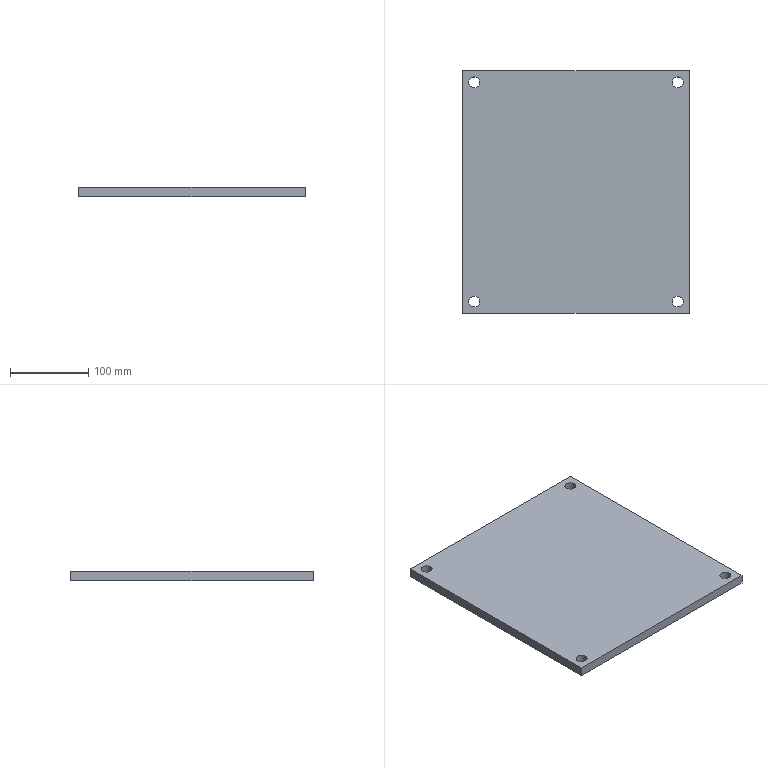Part | STEP file | X77-03027 | 1 solid | 14 faces | box 290 x 310 x 12 mm | volume 1071411 mm3 | cylinder 8 | plane 6 | commonest cylinder face diameters 14 x8
STEP:
#1=CARTESIAN_POINT('',(-3500.936,-1699.184,12.));
#2=VERTEX_POINT('',#1);
#3=CARTESIAN_POINT('',(-3514.936,-1699.184,12.));
#4=VERTEX_POINT('',#3);
#5=CARTESIAN_POINT('',(-3507.936,-1699.184,12.));
#6=DIRECTION('',(0.,0.,-1.));
#7=DIRECTION('',(-1.,0.,0.));
#8=AXIS2_PLACEMENT_3D('',#5,#6,#7);
#9=CIRCLE('',#8,7.);
#10=EDGE_CURVE('',#2,#4,#9,.T.);
#11=ORIENTED_EDGE('',*,*,#10,.F.);
#12=CARTESIAN_POINT('',(-3500.936,-1699.184,0.));
#13=VERTEX_POINT('',#12);
#14=CARTESIAN_POINT('',(-3500.936,-1699.184,0.));
#15=DIRECTION('',(0.,0.,-1.));
#16=VECTOR('',#15,1000.);
#17=LINE('',#14,#16);
#18=EDGE_CURVE('',#2,#13,#17,.T.);
#19=ORIENTED_EDGE('',*,*,#18,.T.);
#20=CARTESIAN_POINT('',(-3514.936,-1699.184,0.));
#21=VERTEX_POINT('',#20);
#22=CARTESIAN_POINT('',(-3507.936,-1699.184,0.));
#23=DIRECTION('',(0.,0.,-1.));
#24=DIRECTION('',(-1.,0.,0.));
#25=AXIS2_PLACEMENT_3D('',#22,#23,#24);
#26=CIRCLE('',#25,7.);
#27=EDGE_CURVE('',#13,#21,#26,.T.);
#28=ORIENTED_EDGE('',*,*,#27,.T.);
#29=CARTESIAN_POINT('',(-3514.936,-1699.184,0.));
#30=DIRECTION('',(0.,0.,-1.));
#31=VECTOR('',#30,1000.);
#32=LINE('',#29,#31);
#33=EDGE_CURVE('',#4,#21,#32,.T.);
#34=ORIENTED_EDGE('',*,*,#33,.F.);
#35=EDGE_LOOP('',(#11,#19,#28,#34));
#36=FACE_OUTER_BOUND('',#35,.T.);
#37=CARTESIAN_POINT('',(-3507.936,-1699.184,0.));
#38=DIRECTION('',(0.,0.,-1.));
#39=DIRECTION('',(-1.,0.,0.));
#40=AXIS2_PLACEMENT_3D('',#37,#38,#39);
#41=CYLINDRICAL_SURFACE('',#40,7.);
#42=ADVANCED_FACE('',(#36),#41,.F.);
#43=CARTESIAN_POINT('',(-3240.936,-1699.184,12.));
#44=VERTEX_POINT('',#43);
#45=CARTESIAN_POINT('',(-3254.936,-1699.184,12.));
#46=VERTEX_POINT('',#45);
#47=CARTESIAN_POINT('',(-3247.936,-1699.184,12.));
#48=DIRECTION('',(0.,0.,-1.));
#49=DIRECTION('',(-1.,0.,0.));
#50=AXIS2_PLACEMENT_3D('',#47,#48,#49);
#51=CIRCLE('',#50,7.);
#52=EDGE_CURVE('',#44,#46,#51,.T.);
#53=ORIENTED_EDGE('',*,*,#52,.F.);
#54=CARTESIAN_POINT('',(-3240.936,-1699.184,0.));
#55=VERTEX_POINT('',#54);
#56=CARTESIAN_POINT('',(-3240.936,-1699.184,0.));
#57=DIRECTION('',(0.,0.,-1.));
#58=VECTOR('',#57,1000.);
#59=LINE('',#56,#58);
#60=EDGE_CURVE('',#44,#55,#59,.T.);
#61=ORIENTED_EDGE('',*,*,#60,.T.);
#62=CARTESIAN_POINT('',(-3254.936,-1699.184,0.));
#63=VERTEX_POINT('',#62);
#64=CARTESIAN_POINT('',(-3247.936,-1699.184,0.));
#65=DIRECTION('',(0.,0.,-1.));
#66=DIRECTION('',(-1.,0.,0.));
#67=AXIS2_PLACEMENT_3D('',#64,#65,#66);
#68=CIRCLE('',#67,7.);
#69=EDGE_CURVE('',#55,#63,#68,.T.);
#70=ORIENTED_EDGE('',*,*,#69,.T.);
#71=CARTESIAN_POINT('',(-3254.936,-1699.184,0.));
#72=DIRECTION('',(0.,0.,-1.));
#73=VECTOR('',#72,1000.);
#74=LINE('',#71,#73);
#75=EDGE_CURVE('',#46,#63,#74,.T.);
#76=ORIENTED_EDGE('',*,*,#75,.F.);
#77=EDGE_LOOP('',(#53,#61,#70,#76));
#78=FACE_OUTER_BOUND('',#77,.T.);
#79=CARTESIAN_POINT('',(-3247.936,-1699.184,0.));
#80=DIRECTION('',(0.,0.,-1.));
#81=DIRECTION('',(-1.,0.,0.));
#82=AXIS2_PLACEMENT_3D('',#79,#80,#81);
#83=CYLINDRICAL_SURFACE('',#82,7.);
#84=ADVANCED_FACE('',(#78),#83,.F.);
#85=CARTESIAN_POINT('',(-3500.936,-1419.184,12.));
#86=VERTEX_POINT('',#85);
#87=CARTESIAN_POINT('',(-3514.936,-1419.184,12.));
#88=VERTEX_POINT('',#87);
#89=CARTESIAN_POINT('',(-3507.936,-1419.184,12.));
#90=DIRECTION('',(0.,0.,-1.));
#91=DIRECTION('',(-1.,0.,0.));
#92=AXIS2_PLACEMENT_3D('',#89,#90,#91);
#93=CIRCLE('',#92,7.);
#94=EDGE_CURVE('',#86,#88,#93,.T.);
#95=ORIENTED_EDGE('',*,*,#94,.F.);
#96=CARTESIAN_POINT('',(-3500.936,-1419.184,0.));
#97=VERTEX_POINT('',#96);
#98=CARTESIAN_POINT('',(-3500.936,-1419.184,0.));
#99=DIRECTION('',(0.,0.,-1.));
#100=VECTOR('',#99,1000.);
#101=LINE('',#98,#100);
#102=EDGE_CURVE('',#86,#97,#101,.T.);
#103=ORIENTED_EDGE('',*,*,#102,.T.);
#104=CARTESIAN_POINT('',(-3514.936,-1419.184,0.));
#105=VERTEX_POINT('',#104);
#106=CARTESIAN_POINT('',(-3507.936,-1419.184,0.));
#107=DIRECTION('',(0.,0.,-1.));
#108=DIRECTION('',(-1.,0.,0.));
#109=AXIS2_PLACEMENT_3D('',#106,#107,#108);
#110=CIRCLE('',#109,7.);
#111=EDGE_CURVE('',#97,#105,#110,.T.);
#112=ORIENTED_EDGE('',*,*,#111,.T.);
#113=CARTESIAN_POINT('',(-3514.936,-1419.184,0.));
#114=DIRECTION('',(0.,0.,-1.));
#115=VECTOR('',#114,1000.);
#116=LINE('',#113,#115);
#117=EDGE_CURVE('',#88,#105,#116,.T.);
#118=ORIENTED_EDGE('',*,*,#117,.F.);
#119=EDGE_LOOP('',(#95,#103,#112,#118));
#120=FACE_OUTER_BOUND('',#119,.T.);
#121=CARTESIAN_POINT('',(-3507.936,-1419.184,0.));
#122=DIRECTION('',(0.,0.,-1.));
#123=DIRECTION('',(-1.,0.,0.));
#124=AXIS2_PLACEMENT_3D('',#121,#122,#123);
#125=CYLINDRICAL_SURFACE('',#124,7.);
#126=ADVANCED_FACE('',(#120),#125,.F.);
#127=CARTESIAN_POINT('',(-3240.936,-1419.184,12.));
#128=VERTEX_POINT('',#127);
#129=CARTESIAN_POINT('',(-3254.936,-1419.184,12.));
#130=VERTEX_POINT('',#129);
#131=CARTESIAN_POINT('',(-3247.936,-1419.184,12.));
#132=DIRECTION('',(0.,0.,-1.));
#133=DIRECTION('',(-1.,0.,0.));
#134=AXIS2_PLACEMENT_3D('',#131,#132,#133);
#135=CIRCLE('',#134,7.);
#136=EDGE_CURVE('',#128,#130,#135,.T.);
#137=ORIENTED_EDGE('',*,*,#136,.F.);
#138=CARTESIAN_POINT('',(-3240.936,-1419.184,0.));
#139=VERTEX_POINT('',#138);
#140=CARTESIAN_POINT('',(-3240.936,-1419.184,0.));
#141=DIRECTION('',(0.,0.,-1.));
#142=VECTOR('',#141,1000.);
#143=LINE('',#140,#142);
#144=EDGE_CURVE('',#128,#139,#143,.T.);
#145=ORIENTED_EDGE('',*,*,#144,.T.);
#146=CARTESIAN_POINT('',(-3254.936,-1419.184,0.));
#147=VERTEX_POINT('',#146);
#148=CARTESIAN_POINT('',(-3247.936,-1419.184,0.));
#149=DIRECTION('',(0.,0.,-1.));
#150=DIRECTION('',(-1.,0.,0.));
#151=AXIS2_PLACEMENT_3D('',#148,#149,#150);
#152=CIRCLE('',#151,7.);
#153=EDGE_CURVE('',#139,#147,#152,.T.);
#154=ORIENTED_EDGE('',*,*,#153,.T.);
#155=CARTESIAN_POINT('',(-3254.936,-1419.184,0.));
#156=DIRECTION('',(0.,0.,-1.));
#157=VECTOR('',#156,1000.);
#158=LINE('',#155,#157);
#159=EDGE_CURVE('',#130,#147,#158,.T.);
#160=ORIENTED_EDGE('',*,*,#159,.F.);
#161=EDGE_LOOP('',(#137,#145,#154,#160));
#162=FACE_OUTER_BOUND('',#161,.T.);
#163=CARTESIAN_POINT('',(-3247.936,-1419.184,0.));
#164=DIRECTION('',(0.,0.,-1.));
#165=DIRECTION('',(-1.,0.,0.));
#166=AXIS2_PLACEMENT_3D('',#163,#164,#165);
#167=CYLINDRICAL_SURFACE('',#166,7.);
#168=ADVANCED_FACE('',(#162),#167,.F.);
#169=CARTESIAN_POINT('',(-3232.936,-1404.184,0.));
#170=VERTEX_POINT('',#169);
#171=CARTESIAN_POINT('',(-3522.936,-1404.184,0.));
#172=VERTEX_POINT('',#171);
#173=CARTESIAN_POINT('',(-3522.936,-1404.184,0.));
#174=DIRECTION('',(-1.,0.,0.));
#175=VECTOR('',#174,1000.);
#176=LINE('',#173,#175);
#177=EDGE_CURVE('',#170,#172,#176,.T.);
#178=ORIENTED_EDGE('',*,*,#177,.T.);
#179=CARTESIAN_POINT('',(-3522.936,-1404.184,12.));
#180=VERTEX_POINT('',#179);
#181=CARTESIAN_POINT('',(-3522.936,-1404.184,12.));
#182=DIRECTION('',(0.,0.,-1.));
#183=VECTOR('',#182,1000.);
#184=LINE('',#181,#183);
#185=EDGE_CURVE('',#180,#172,#184,.T.);
#186=ORIENTED_EDGE('',*,*,#185,.F.);
#187=CARTESIAN_POINT('',(-3232.936,-1404.184,12.));
#188=VERTEX_POINT('',#187);
#189=CARTESIAN_POINT('',(-3522.936,-1404.184,12.));
#190=DIRECTION('',(-1.,0.,0.));
#191=VECTOR('',#190,1000.);
#192=LINE('',#189,#191);
#193=EDGE_CURVE('',#188,#180,#192,.T.);
#194=ORIENTED_EDGE('',*,*,#193,.F.);
#195=CARTESIAN_POINT('',(-3232.936,-1404.184,12.));
#196=DIRECTION('',(0.,0.,-1.));
#197=VECTOR('',#196,1000.);
#198=LINE('',#195,#197);
#199=EDGE_CURVE('',#188,#170,#198,.T.);
#200=ORIENTED_EDGE('',*,*,#199,.T.);
#201=EDGE_LOOP('',(#178,#186,#194,#200));
#202=FACE_OUTER_BOUND('',#201,.T.);
#203=CARTESIAN_POINT('',(-3522.936,-1404.184,12.));
#204=DIRECTION('',(0.,-1.,0.));
#205=DIRECTION('',(0.,0.,-1.));
#206=AXIS2_PLACEMENT_3D('',#203,#204,#205);
#207=PLANE('',#206);
#208=ADVANCED_FACE('',(#202),#207,.F.);
#209=CARTESIAN_POINT('',(-3522.936,-1714.184,0.));
#210=VERTEX_POINT('',#209);
#211=CARTESIAN_POINT('',(-3522.936,-1404.184,0.));
#212=DIRECTION('',(0.,-1.,0.));
#213=VECTOR('',#212,1000.);
#214=LINE('',#211,#213);
#215=EDGE_CURVE('',#172,#210,#214,.T.);
#216=ORIENTED_EDGE('',*,*,#215,.T.);
#217=CARTESIAN_POINT('',(-3522.936,-1714.184,12.));
#218=VERTEX_POINT('',#217);
#219=CARTESIAN_POINT('',(-3522.936,-1714.184,12.));
#220=DIRECTION('',(0.,0.,-1.));
#221=VECTOR('',#220,1000.);
#222=LINE('',#219,#221);
#223=EDGE_CURVE('',#218,#210,#222,.T.);
#224=ORIENTED_EDGE('',*,*,#223,.F.);
#225=CARTESIAN_POINT('',(-3522.936,-1404.184,12.));
#226=DIRECTION('',(0.,-1.,0.));
#227=VECTOR('',#226,1000.);
#228=LINE('',#225,#227);
#229=EDGE_CURVE('',#180,#218,#228,.T.);
#230=ORIENTED_EDGE('',*,*,#229,.F.);
#231=ORIENTED_EDGE('',*,*,#185,.T.);
#232=EDGE_LOOP('',(#216,#224,#230,#231));
#233=FACE_OUTER_BOUND('',#232,.T.);
#234=CARTESIAN_POINT('',(-3522.936,-1404.184,12.));
#235=DIRECTION('',(1.,0.,0.));
#236=DIRECTION('',(0.,0.,-1.));
#237=AXIS2_PLACEMENT_3D('',#234,#235,#236);
#238=PLANE('',#237);
#239=ADVANCED_FACE('',(#233),#238,.F.);
#240=CARTESIAN_POINT('',(-3232.936,-1714.184,0.));
#241=VERTEX_POINT('',#240);
#242=CARTESIAN_POINT('',(-3522.936,-1714.184,0.));
#243=DIRECTION('',(1.,0.,0.));
#244=VECTOR('',#243,1000.);
#245=LINE('',#242,#244);
#246=EDGE_CURVE('',#210,#241,#245,.T.);
#247=ORIENTED_EDGE('',*,*,#246,.T.);
#248=CARTESIAN_POINT('',(-3232.936,-1714.184,12.));
#249=VERTEX_POINT('',#248);
#250=CARTESIAN_POINT('',(-3232.936,-1714.184,12.));
#251=DIRECTION('',(0.,0.,-1.));
#252=VECTOR('',#251,1000.);
#253=LINE('',#250,#252);
#254=EDGE_CURVE('',#249,#241,#253,.T.);
#255=ORIENTED_EDGE('',*,*,#254,.F.);
#256=CARTESIAN_POINT('',(-3522.936,-1714.184,12.));
#257=DIRECTION('',(1.,0.,0.));
#258=VECTOR('',#257,1000.);
#259=LINE('',#256,#258);
#260=EDGE_CURVE('',#218,#249,#259,.T.);
#261=ORIENTED_EDGE('',*,*,#260,.F.);
#262=ORIENTED_EDGE('',*,*,#223,.T.);
#263=EDGE_LOOP('',(#247,#255,#261,#262));
#264=FACE_OUTER_BOUND('',#263,.T.);
#265=CARTESIAN_POINT('',(-3522.936,-1714.184,12.));
#266=DIRECTION('',(0.,1.,0.));
#267=DIRECTION('',(0.,0.,1.));
#268=AXIS2_PLACEMENT_3D('',#265,#266,#267);
#269=PLANE('',#268);
#270=ADVANCED_FACE('',(#264),#269,.F.);
#271=CARTESIAN_POINT('',(-3232.936,-1404.184,0.));
#272=DIRECTION('',(0.,1.,0.));
#273=VECTOR('',#272,1000.);
#274=LINE('',#271,#273);
#275=EDGE_CURVE('',#241,#170,#274,.T.);
#276=ORIENTED_EDGE('',*,*,#275,.T.);
#277=ORIENTED_EDGE('',*,*,#199,.F.);
#278=CARTESIAN_POINT('',(-3232.936,-1404.184,12.));
#279=DIRECTION('',(0.,1.,0.));
#280=VECTOR('',#279,1000.);
#281=LINE('',#278,#280);
#282=EDGE_CURVE('',#249,#188,#281,.T.);
#283=ORIENTED_EDGE('',*,*,#282,.F.);
#284=ORIENTED_EDGE('',*,*,#254,.T.);
#285=EDGE_LOOP('',(#276,#277,#283,#284));
#286=FACE_OUTER_BOUND('',#285,.T.);
#287=CARTESIAN_POINT('',(-3232.936,-1404.184,12.));
#288=DIRECTION('',(-1.,0.,0.));
#289=DIRECTION('',(0.,0.,1.));
#290=AXIS2_PLACEMENT_3D('',#287,#288,#289);
#291=PLANE('',#290);
#292=ADVANCED_FACE('',(#286),#291,.F.);
#293=CARTESIAN_POINT('',(-3507.936,-1699.184,12.));
#294=DIRECTION('',(0.,0.,-1.));
#295=DIRECTION('',(-1.,0.,0.));
#296=AXIS2_PLACEMENT_3D('',#293,#294,#295);
#297=CIRCLE('',#296,7.);
#298=EDGE_CURVE('',#4,#2,#297,.T.);
#299=ORIENTED_EDGE('',*,*,#298,.T.);
#300=ORIENTED_EDGE('',*,*,#10,.T.);
#301=EDGE_LOOP('',(#299,#300));
#302=FACE_BOUND('',#301,.T.);
#303=CARTESIAN_POINT('',(-3247.936,-1699.184,12.));
#304=DIRECTION('',(0.,0.,-1.));
#305=DIRECTION('',(-1.,0.,0.));
#306=AXIS2_PLACEMENT_3D('',#303,#304,#305);
#307=CIRCLE('',#306,7.);
#308=EDGE_CURVE('',#46,#44,#307,.T.);
#309=ORIENTED_EDGE('',*,*,#308,.T.);
#310=ORIENTED_EDGE('',*,*,#52,.T.);
#311=EDGE_LOOP('',(#309,#310));
#312=FACE_BOUND('',#311,.T.);
#313=CARTESIAN_POINT('',(-3507.936,-1419.184,12.));
#314=DIRECTION('',(0.,0.,-1.));
#315=DIRECTION('',(-1.,0.,0.));
#316=AXIS2_PLACEMENT_3D('',#313,#314,#315);
#317=CIRCLE('',#316,7.);
#318=EDGE_CURVE('',#88,#86,#317,.T.);
#319=ORIENTED_EDGE('',*,*,#318,.T.);
#320=ORIENTED_EDGE('',*,*,#94,.T.);
#321=EDGE_LOOP('',(#319,#320));
#322=FACE_BOUND('',#321,.T.);
#323=CARTESIAN_POINT('',(-3247.936,-1419.184,12.));
#324=DIRECTION('',(0.,0.,-1.));
#325=DIRECTION('',(-1.,0.,0.));
#326=AXIS2_PLACEMENT_3D('',#323,#324,#325);
#327=CIRCLE('',#326,7.);
#328=EDGE_CURVE('',#130,#128,#327,.T.);
#329=ORIENTED_EDGE('',*,*,#328,.T.);
#330=ORIENTED_EDGE('',*,*,#136,.T.);
#331=EDGE_LOOP('',(#329,#330));
#332=FACE_BOUND('',#331,.T.);
#333=ORIENTED_EDGE('',*,*,#193,.T.);
#334=ORIENTED_EDGE('',*,*,#229,.T.);
#335=ORIENTED_EDGE('',*,*,#260,.T.);
#336=ORIENTED_EDGE('',*,*,#282,.T.);
#337=EDGE_LOOP('',(#333,#334,#335,#336));
#338=FACE_OUTER_BOUND('',#337,.T.);
#339=CARTESIAN_POINT('',(-3232.936,-1404.184,12.));
#340=DIRECTION('',(0.,0.,-1.));
#341=DIRECTION('',(-1.,0.,0.));
#342=AXIS2_PLACEMENT_3D('',#339,#340,#341);
#343=PLANE('',#342);
#344=ADVANCED_FACE('',(#302,#312,#322,#332,#338),#343,.F.);
#345=CARTESIAN_POINT('',(-3507.936,-1699.184,0.));
#346=DIRECTION('',(0.,0.,-1.));
#347=DIRECTION('',(-1.,0.,0.));
#348=AXIS2_PLACEMENT_3D('',#345,#346,#347);
#349=CIRCLE('',#348,7.);
#350=EDGE_CURVE('',#21,#13,#349,.T.);
#351=ORIENTED_EDGE('',*,*,#350,.F.);
#352=ORIENTED_EDGE('',*,*,#27,.F.);
#353=EDGE_LOOP('',(#351,#352));
#354=FACE_BOUND('',#353,.T.);
#355=CARTESIAN_POINT('',(-3247.936,-1699.184,0.));
#356=DIRECTION('',(0.,0.,-1.));
#357=DIRECTION('',(-1.,0.,0.));
#358=AXIS2_PLACEMENT_3D('',#355,#356,#357);
#359=CIRCLE('',#358,7.);
#360=EDGE_CURVE('',#63,#55,#359,.T.);
#361=ORIENTED_EDGE('',*,*,#360,.F.);
#362=ORIENTED_EDGE('',*,*,#69,.F.);
#363=EDGE_LOOP('',(#361,#362));
#364=FACE_BOUND('',#363,.T.);
#365=CARTESIAN_POINT('',(-3507.936,-1419.184,0.));
#366=DIRECTION('',(0.,0.,-1.));
#367=DIRECTION('',(-1.,0.,0.));
#368=AXIS2_PLACEMENT_3D('',#365,#366,#367);
#369=CIRCLE('',#368,7.);
#370=EDGE_CURVE('',#105,#97,#369,.T.);
#371=ORIENTED_EDGE('',*,*,#370,.F.);
#372=ORIENTED_EDGE('',*,*,#111,.F.);
#373=EDGE_LOOP('',(#371,#372));
#374=FACE_BOUND('',#373,.T.);
#375=CARTESIAN_POINT('',(-3247.936,-1419.184,0.));
#376=DIRECTION('',(0.,0.,-1.));
#377=DIRECTION('',(-1.,0.,0.));
#378=AXIS2_PLACEMENT_3D('',#375,#376,#377);
#379=CIRCLE('',#378,7.);
#380=EDGE_CURVE('',#147,#139,#379,.T.);
#381=ORIENTED_EDGE('',*,*,#380,.F.);
#382=ORIENTED_EDGE('',*,*,#153,.F.);
#383=EDGE_LOOP('',(#381,#382));
#384=FACE_BOUND('',#383,.T.);
#385=ORIENTED_EDGE('',*,*,#177,.F.);
#386=ORIENTED_EDGE('',*,*,#275,.F.);
#387=ORIENTED_EDGE('',*,*,#246,.F.);
#388=ORIENTED_EDGE('',*,*,#215,.F.);
#389=EDGE_LOOP('',(#385,#386,#387,#388));
#390=FACE_OUTER_BOUND('',#389,.T.);
#391=CARTESIAN_POINT('',(-3232.936,-1404.184,0.));
#392=DIRECTION('',(0.,0.,-1.));
#393=DIRECTION('',(-1.,0.,0.));
#394=AXIS2_PLACEMENT_3D('',#391,#392,#393);
#395=PLANE('',#394);
#396=ADVANCED_FACE('',(#354,#364,#374,#384,#390),#395,.T.);
#397=ORIENTED_EDGE('',*,*,#144,.F.);
#398=ORIENTED_EDGE('',*,*,#328,.F.);
#399=ORIENTED_EDGE('',*,*,#159,.T.);
#400=ORIENTED_EDGE('',*,*,#380,.T.);
#401=EDGE_LOOP('',(#397,#398,#399,#400));
#402=FACE_OUTER_BOUND('',#401,.T.);
#403=CARTESIAN_POINT('',(-3247.936,-1419.184,0.));
#404=DIRECTION('',(0.,0.,-1.));
#405=DIRECTION('',(-1.,0.,0.));
#406=AXIS2_PLACEMENT_3D('',#403,#404,#405);
#407=CYLINDRICAL_SURFACE('',#406,7.);
#408=ADVANCED_FACE('',(#402),#407,.F.);
#409=ORIENTED_EDGE('',*,*,#102,.F.);
#410=ORIENTED_EDGE('',*,*,#318,.F.);
#411=ORIENTED_EDGE('',*,*,#117,.T.);
#412=ORIENTED_EDGE('',*,*,#370,.T.);
#413=EDGE_LOOP('',(#409,#410,#411,#412));
#414=FACE_OUTER_BOUND('',#413,.T.);
#415=CARTESIAN_POINT('',(-3507.936,-1419.184,0.));
#416=DIRECTION('',(0.,0.,-1.));
#417=DIRECTION('',(-1.,0.,0.));
#418=AXIS2_PLACEMENT_3D('',#415,#416,#417);
#419=CYLINDRICAL_SURFACE('',#418,7.);
#420=ADVANCED_FACE('',(#414),#419,.F.);
#421=ORIENTED_EDGE('',*,*,#60,.F.);
#422=ORIENTED_EDGE('',*,*,#308,.F.);
#423=ORIENTED_EDGE('',*,*,#75,.T.);
#424=ORIENTED_EDGE('',*,*,#360,.T.);
#425=EDGE_LOOP('',(#421,#422,#423,#424));
#426=FACE_OUTER_BOUND('',#425,.T.);
#427=CARTESIAN_POINT('',(-3247.936,-1699.184,0.));
#428=DIRECTION('',(0.,0.,-1.));
#429=DIRECTION('',(-1.,0.,0.));
#430=AXIS2_PLACEMENT_3D('',#427,#428,#429);
#431=CYLINDRICAL_SURFACE('',#430,7.);
#432=ADVANCED_FACE('',(#426),#431,.F.);
#433=ORIENTED_EDGE('',*,*,#18,.F.);
#434=ORIENTED_EDGE('',*,*,#298,.F.);
#435=ORIENTED_EDGE('',*,*,#33,.T.);
#436=ORIENTED_EDGE('',*,*,#350,.T.);
#437=EDGE_LOOP('',(#433,#434,#435,#436));
#438=FACE_OUTER_BOUND('',#437,.T.);
#439=CARTESIAN_POINT('',(-3507.936,-1699.184,0.));
#440=DIRECTION('',(0.,0.,-1.));
#441=DIRECTION('',(-1.,0.,0.));
#442=AXIS2_PLACEMENT_3D('',#439,#440,#441);
#443=CYLINDRICAL_SURFACE('',#442,7.);
#444=ADVANCED_FACE('',(#438),#443,.F.);
#445=CLOSED_SHELL('',(#42,#84,#126,#168,#208,#239,#270,#292,#344,#396,#408,#420,#432,#444));
#446=MANIFOLD_SOLID_BREP('',#445);
#447=CARTESIAN_POINT('',(0.,0.,0.));
#448=DIRECTION('',(0.,0.,1.));
#449=DIRECTION('',(1.,0.,0.));
#450=AXIS2_PLACEMENT_3D('',#447,#448,#449);
#451=(LENGTH_UNIT()NAMED_UNIT(*)SI_UNIT(.MILLI.,.METRE.));
#452=UNCERTAINTY_MEASURE_WITH_UNIT(LENGTH_MEASURE(0.00001),#451,'','');
#453=(NAMED_UNIT(*)PLANE_ANGLE_UNIT()SI_UNIT($,.RADIAN.));
#454=(NAMED_UNIT(*)SI_UNIT($,.STERADIAN.)SOLID_ANGLE_UNIT());
#455=(GEOMETRIC_REPRESENTATION_CONTEXT(3)GLOBAL_UNCERTAINTY_ASSIGNED_CONTEXT((#452))GLOBAL_UNIT_ASSIGNED_CONTEXT((#451,#453,#454))REPRESENTATION_CONTEXT('',''));
#456=ADVANCED_BREP_SHAPE_REPRESENTATION('',(#446,#450),#455);